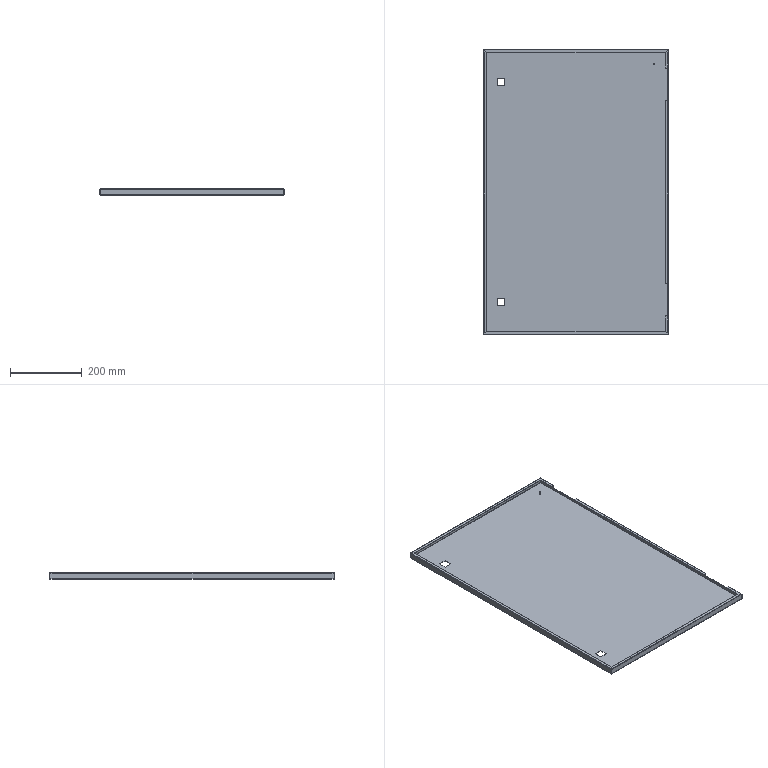Part | STEP file | 1 solid | 129 faces | box 515 x 796 x 17 mm | volume 556251 mm3 | plane 95 | cylinder 26 | spline 8 | commonest cylinder face diameters 0.02 x10 2.42 x10 2 x4 3 x2